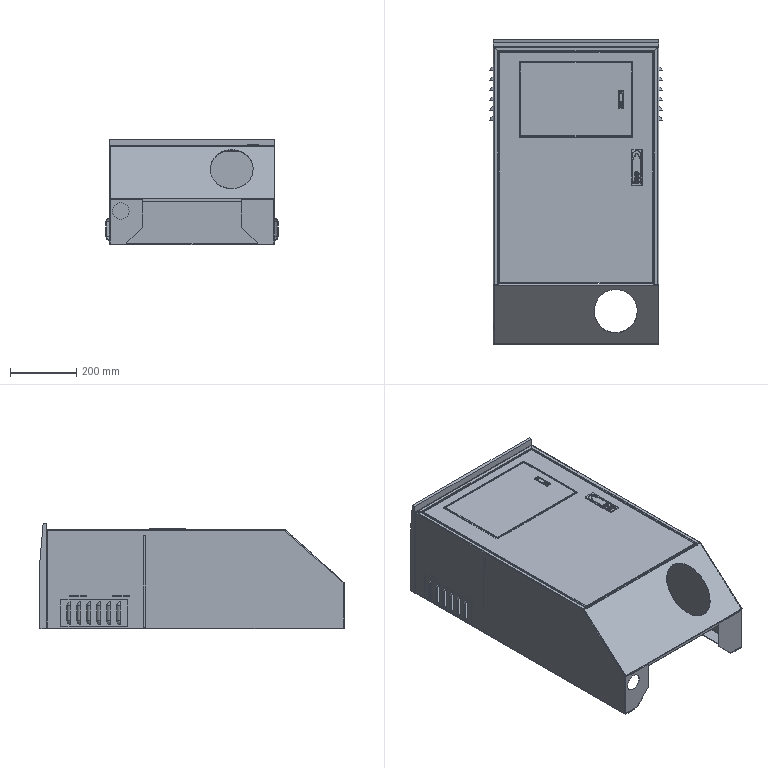Part | SolidWorks | features InContextFeatHolder 2 | 19 solids | 1164 faces | box 520 x 920 x 319.997 mm | volume 6570455 mm3 | plane 587 | cylinder 320 | spline 121 | sphere 64 | torus 48 | cone 24 | commonest cylinder face diameters 1.473 x38 5.473 x38 4 x36 2 x34 20 x24 1 x22